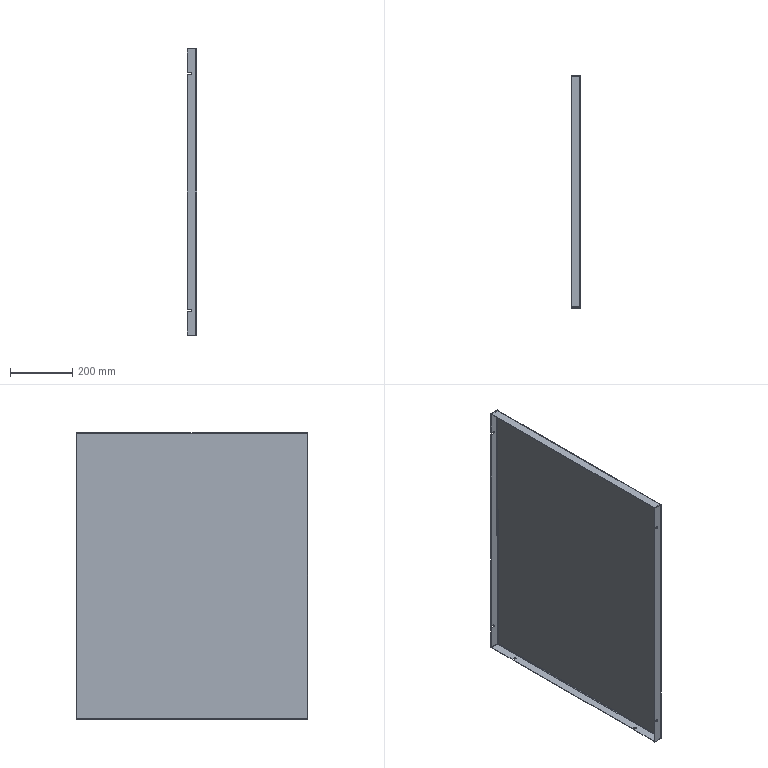Part | STEP file | FB-6_1-2 | 1 solid | 58 faces | box 30 x 748 x 923 mm | volume 1172313 mm3 | plane 44 | cylinder 14 | commonest cylinder face diameters 7 x6 3 x4 6 x4